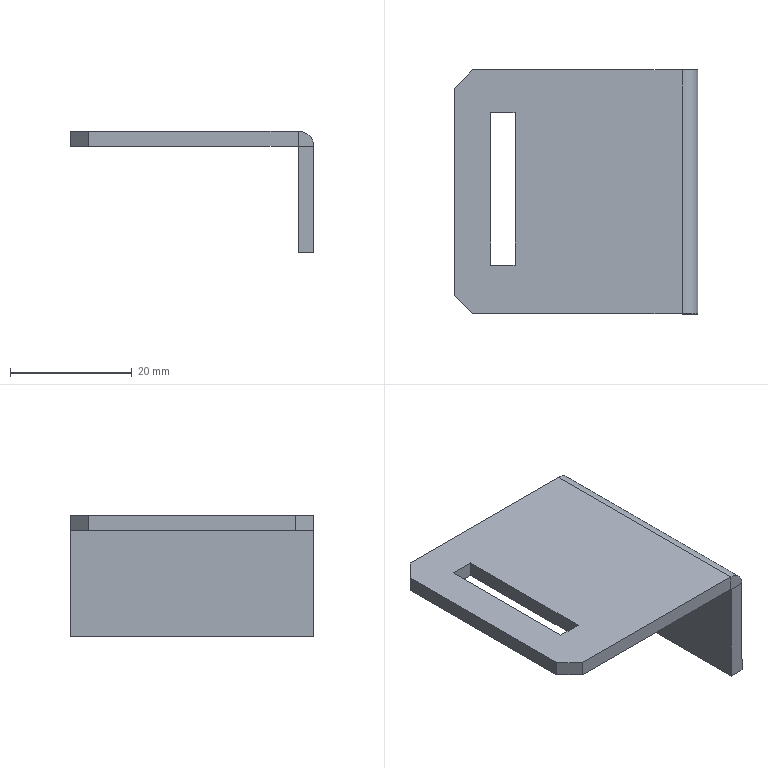Part | SolidWorks | features Chamfer 1, EdgeFlange 1, FlatPattern 1, ICE 1, SMBaseFlange 1, SheetMetal 1 | 1 solid | 20 faces | box 40 x 40 x 20 mm | volume 5420 mm3 | plane 18 | cylinder 2 | commonest cylinder face diameters 0.2 x1 5.2 x1
STEP:
#1=CARTESIAN_POINT('',(-17.,-20.,0.));
#2=VERTEX_POINT('',#1);
#3=CARTESIAN_POINT('',(17.4,-20.,0.));
#4=VERTEX_POINT('',#3);
#5=CARTESIAN_POINT('',(-20.,-20.,0.));
#6=DIRECTION('',(1.,0.,0.));
#7=VECTOR('',#6,1000.);
#8=LINE('',#5,#7);
#9=EDGE_CURVE('',#2,#4,#8,.T.);
#10=ORIENTED_EDGE('',*,*,#9,.F.);
#11=CARTESIAN_POINT('',(-17.,-20.,-2.5));
#12=VERTEX_POINT('',#11);
#13=CARTESIAN_POINT('',(-17.,-20.,-2.5));
#14=DIRECTION('',(0.,0.,-1.));
#15=VECTOR('',#14,1000.);
#16=LINE('',#13,#15);
#17=EDGE_CURVE('',#2,#12,#16,.T.);
#18=ORIENTED_EDGE('',*,*,#17,.T.);
#19=CARTESIAN_POINT('',(17.4,-20.,-2.5));
#20=VERTEX_POINT('',#19);
#21=CARTESIAN_POINT('',(-20.,-20.,-2.5));
#22=DIRECTION('',(1.,0.,0.));
#23=VECTOR('',#22,1000.);
#24=LINE('',#21,#23);
#25=EDGE_CURVE('',#12,#20,#24,.T.);
#26=ORIENTED_EDGE('',*,*,#25,.T.);
#27=CARTESIAN_POINT('',(17.4,-20.,-2.5));
#28=DIRECTION('',(0.,0.,1.));
#29=VECTOR('',#28,1000.);
#30=LINE('',#27,#29);
#31=EDGE_CURVE('',#20,#4,#30,.T.);
#32=ORIENTED_EDGE('',*,*,#31,.T.);
#33=EDGE_LOOP('',(#10,#18,#26,#32));
#34=FACE_OUTER_BOUND('',#33,.T.);
#35=CARTESIAN_POINT('',(-20.,-20.,-2.5));
#36=DIRECTION('',(0.,-1.,0.));
#37=DIRECTION('',(0.,0.,-1.));
#38=AXIS2_PLACEMENT_3D('',#35,#36,#37);
#39=PLANE('',#38);
#40=ADVANCED_FACE('',(#34),#39,.T.);
#41=CARTESIAN_POINT('',(-14.,-12.,-2.5));
#42=VERTEX_POINT('',#41);
#43=CARTESIAN_POINT('',(-10.,-12.,-2.5));
#44=VERTEX_POINT('',#43);
#45=CARTESIAN_POINT('',(0.,-12.,-2.5));
#46=DIRECTION('',(1.,0.,0.));
#47=VECTOR('',#46,1000.);
#48=LINE('',#45,#47);
#49=EDGE_CURVE('',#42,#44,#48,.T.);
#50=ORIENTED_EDGE('',*,*,#49,.T.);
#51=CARTESIAN_POINT('',(-10.,13.,-2.5));
#52=VERTEX_POINT('',#51);
#53=CARTESIAN_POINT('',(-10.,0.,-2.5));
#54=DIRECTION('',(0.,1.,0.));
#55=VECTOR('',#54,1000.);
#56=LINE('',#53,#55);
#57=EDGE_CURVE('',#44,#52,#56,.T.);
#58=ORIENTED_EDGE('',*,*,#57,.T.);
#59=CARTESIAN_POINT('',(-14.,13.,-2.5));
#60=VERTEX_POINT('',#59);
#61=CARTESIAN_POINT('',(0.,13.,-2.5));
#62=DIRECTION('',(-1.,0.,0.));
#63=VECTOR('',#62,1000.);
#64=LINE('',#61,#63);
#65=EDGE_CURVE('',#52,#60,#64,.T.);
#66=ORIENTED_EDGE('',*,*,#65,.T.);
#67=CARTESIAN_POINT('',(-14.,0.,-2.5));
#68=DIRECTION('',(0.,-1.,0.));
#69=VECTOR('',#68,1000.);
#70=LINE('',#67,#69);
#71=EDGE_CURVE('',#60,#42,#70,.T.);
#72=ORIENTED_EDGE('',*,*,#71,.T.);
#73=EDGE_LOOP('',(#50,#58,#66,#72));
#74=FACE_BOUND('',#73,.T.);
#75=CARTESIAN_POINT('',(-20.,17.,-2.5));
#76=VERTEX_POINT('',#75);
#77=CARTESIAN_POINT('',(-20.,-17.,-2.5));
#78=VERTEX_POINT('',#77);
#79=CARTESIAN_POINT('',(-20.,20.,-2.5));
#80=DIRECTION('',(0.,-1.,0.));
#81=VECTOR('',#80,1000.);
#82=LINE('',#79,#81);
#83=EDGE_CURVE('',#76,#78,#82,.T.);
#84=ORIENTED_EDGE('',*,*,#83,.F.);
#85=CARTESIAN_POINT('',(-17.,20.,-2.5));
#86=VERTEX_POINT('',#85);
#87=CARTESIAN_POINT('',(-17.,20.,-2.5));
#88=DIRECTION('',(0.7071,0.7071,0.));
#89=VECTOR('',#88,1000.);
#90=LINE('',#87,#89);
#91=EDGE_CURVE('',#76,#86,#90,.T.);
#92=ORIENTED_EDGE('',*,*,#91,.T.);
#93=CARTESIAN_POINT('',(17.4,20.,-2.5));
#94=VERTEX_POINT('',#93);
#95=CARTESIAN_POINT('',(-20.,20.,-2.5));
#96=DIRECTION('',(-1.,0.,0.));
#97=VECTOR('',#96,1000.);
#98=LINE('',#95,#97);
#99=EDGE_CURVE('',#94,#86,#98,.T.);
#100=ORIENTED_EDGE('',*,*,#99,.F.);
#101=CARTESIAN_POINT('',(17.4,-20.,-2.5));
#102=DIRECTION('',(0.,1.,0.));
#103=VECTOR('',#102,1000.);
#104=LINE('',#101,#103);
#105=EDGE_CURVE('',#20,#94,#104,.T.);
#106=ORIENTED_EDGE('',*,*,#105,.F.);
#107=ORIENTED_EDGE('',*,*,#25,.F.);
#108=CARTESIAN_POINT('',(-20.,-17.,-2.5));
#109=DIRECTION('',(-0.7071,0.7071,0.));
#110=VECTOR('',#109,1000.);
#111=LINE('',#108,#110);
#112=EDGE_CURVE('',#12,#78,#111,.T.);
#113=ORIENTED_EDGE('',*,*,#112,.T.);
#114=EDGE_LOOP('',(#84,#92,#100,#106,#107,#113));
#115=FACE_OUTER_BOUND('',#114,.T.);
#116=CARTESIAN_POINT('',(0.,0.,-2.5));
#117=DIRECTION('',(0.,0.,1.));
#118=DIRECTION('',(1.,0.,0.));
#119=AXIS2_PLACEMENT_3D('',#116,#117,#118);
#120=PLANE('',#119);
#121=ADVANCED_FACE('',(#74,#115),#120,.F.);
#122=CARTESIAN_POINT('',(-10.,-12.,0.));
#123=VERTEX_POINT('',#122);
#124=CARTESIAN_POINT('',(-10.,13.,0.));
#125=VERTEX_POINT('',#124);
#126=CARTESIAN_POINT('',(-10.,13.,0.));
#127=DIRECTION('',(0.,1.,0.));
#128=VECTOR('',#127,1000.);
#129=LINE('',#126,#128);
#130=EDGE_CURVE('',#123,#125,#129,.T.);
#131=ORIENTED_EDGE('',*,*,#130,.F.);
#132=CARTESIAN_POINT('',(-14.,-12.,0.));
#133=VERTEX_POINT('',#132);
#134=CARTESIAN_POINT('',(-14.,-12.,0.));
#135=DIRECTION('',(1.,0.,0.));
#136=VECTOR('',#135,1000.);
#137=LINE('',#134,#136);
#138=EDGE_CURVE('',#133,#123,#137,.T.);
#139=ORIENTED_EDGE('',*,*,#138,.F.);
#140=CARTESIAN_POINT('',(-14.,13.,0.));
#141=VERTEX_POINT('',#140);
#142=CARTESIAN_POINT('',(-14.,13.,0.));
#143=DIRECTION('',(0.,-1.,0.));
#144=VECTOR('',#143,1000.);
#145=LINE('',#142,#144);
#146=EDGE_CURVE('',#141,#133,#145,.T.);
#147=ORIENTED_EDGE('',*,*,#146,.F.);
#148=CARTESIAN_POINT('',(-14.,13.,0.));
#149=DIRECTION('',(-1.,0.,0.));
#150=VECTOR('',#149,1000.);
#151=LINE('',#148,#150);
#152=EDGE_CURVE('',#125,#141,#151,.T.);
#153=ORIENTED_EDGE('',*,*,#152,.F.);
#154=EDGE_LOOP('',(#131,#139,#147,#153));
#155=FACE_BOUND('',#154,.T.);
#156=CARTESIAN_POINT('',(17.4,20.,0.));
#157=VERTEX_POINT('',#156);
#158=CARTESIAN_POINT('',(-17.,20.,0.));
#159=VERTEX_POINT('',#158);
#160=CARTESIAN_POINT('',(-20.,20.,0.));
#161=DIRECTION('',(-1.,0.,0.));
#162=VECTOR('',#161,1000.);
#163=LINE('',#160,#162);
#164=EDGE_CURVE('',#157,#159,#163,.T.);
#165=ORIENTED_EDGE('',*,*,#164,.T.);
#166=CARTESIAN_POINT('',(-20.,17.,0.));
#167=VERTEX_POINT('',#166);
#168=CARTESIAN_POINT('',(-18.5,18.5,0.));
#169=DIRECTION('',(-0.7071,-0.7071,0.));
#170=VECTOR('',#169,1000.);
#171=LINE('',#168,#170);
#172=EDGE_CURVE('',#159,#167,#171,.T.);
#173=ORIENTED_EDGE('',*,*,#172,.T.);
#174=CARTESIAN_POINT('',(-20.,-17.,0.));
#175=VERTEX_POINT('',#174);
#176=CARTESIAN_POINT('',(-20.,20.,0.));
#177=DIRECTION('',(0.,-1.,0.));
#178=VECTOR('',#177,1000.);
#179=LINE('',#176,#178);
#180=EDGE_CURVE('',#167,#175,#179,.T.);
#181=ORIENTED_EDGE('',*,*,#180,.T.);
#182=CARTESIAN_POINT('',(-18.5,-18.5,0.));
#183=DIRECTION('',(0.7071,-0.7071,0.));
#184=VECTOR('',#183,1000.);
#185=LINE('',#182,#184);
#186=EDGE_CURVE('',#175,#2,#185,.T.);
#187=ORIENTED_EDGE('',*,*,#186,.T.);
#188=ORIENTED_EDGE('',*,*,#9,.T.);
#189=CARTESIAN_POINT('',(17.4,-20.,0.));
#190=DIRECTION('',(0.,1.,0.));
#191=VECTOR('',#190,1000.);
#192=LINE('',#189,#191);
#193=EDGE_CURVE('',#4,#157,#192,.T.);
#194=ORIENTED_EDGE('',*,*,#193,.T.);
#195=EDGE_LOOP('',(#165,#173,#181,#187,#188,#194));
#196=FACE_OUTER_BOUND('',#195,.T.);
#197=CARTESIAN_POINT('',(0.,0.,0.));
#198=DIRECTION('',(0.,0.,1.));
#199=DIRECTION('',(1.,0.,0.));
#200=AXIS2_PLACEMENT_3D('',#197,#198,#199);
#201=PLANE('',#200);
#202=ADVANCED_FACE('',(#155,#196),#201,.T.);
#203=ORIENTED_EDGE('',*,*,#180,.F.);
#204=CARTESIAN_POINT('',(-20.,17.,-2.5));
#205=DIRECTION('',(0.,0.,-1.));
#206=VECTOR('',#205,1000.);
#207=LINE('',#204,#206);
#208=EDGE_CURVE('',#167,#76,#207,.T.);
#209=ORIENTED_EDGE('',*,*,#208,.T.);
#210=ORIENTED_EDGE('',*,*,#83,.T.);
#211=CARTESIAN_POINT('',(-20.,-17.,-2.5));
#212=DIRECTION('',(0.,0.,1.));
#213=VECTOR('',#212,1000.);
#214=LINE('',#211,#213);
#215=EDGE_CURVE('',#78,#175,#214,.T.);
#216=ORIENTED_EDGE('',*,*,#215,.T.);
#217=EDGE_LOOP('',(#203,#209,#210,#216));
#218=FACE_OUTER_BOUND('',#217,.T.);
#219=CARTESIAN_POINT('',(-20.,20.,-2.5));
#220=DIRECTION('',(-1.,0.,0.));
#221=DIRECTION('',(0.,0.,1.));
#222=AXIS2_PLACEMENT_3D('',#219,#220,#221);
#223=PLANE('',#222);
#224=ADVANCED_FACE('',(#218),#223,.T.);
#225=ORIENTED_EDGE('',*,*,#99,.T.);
#226=CARTESIAN_POINT('',(-17.,20.,-2.5));
#227=DIRECTION('',(0.,0.,1.));
#228=VECTOR('',#227,1000.);
#229=LINE('',#226,#228);
#230=EDGE_CURVE('',#86,#159,#229,.T.);
#231=ORIENTED_EDGE('',*,*,#230,.T.);
#232=ORIENTED_EDGE('',*,*,#164,.F.);
#233=CARTESIAN_POINT('',(17.4,20.,-2.5));
#234=DIRECTION('',(0.,0.,1.));
#235=VECTOR('',#234,1000.);
#236=LINE('',#233,#235);
#237=EDGE_CURVE('',#94,#157,#236,.T.);
#238=ORIENTED_EDGE('',*,*,#237,.F.);
#239=EDGE_LOOP('',(#225,#231,#232,#238));
#240=FACE_OUTER_BOUND('',#239,.T.);
#241=CARTESIAN_POINT('',(-20.,20.,-2.5));
#242=DIRECTION('',(0.,1.,0.));
#243=DIRECTION('',(0.,0.,1.));
#244=AXIS2_PLACEMENT_3D('',#241,#242,#243);
#245=PLANE('',#244);
#246=ADVANCED_FACE('',(#240),#245,.T.);
#247=CARTESIAN_POINT('',(17.5,20.,-2.6));
#248=VERTEX_POINT('',#247);
#249=CARTESIAN_POINT('',(20.,20.,-2.6));
#250=VERTEX_POINT('',#249);
#251=CARTESIAN_POINT('',(20.,20.,-2.6));
#252=DIRECTION('',(1.,0.,0.));
#253=VECTOR('',#252,1000.);
#254=LINE('',#251,#253);
#255=EDGE_CURVE('',#248,#250,#254,.T.);
#256=ORIENTED_EDGE('',*,*,#255,.F.);
#257=CARTESIAN_POINT('',(17.4,20.,-2.6));
#258=DIRECTION('',(0.,1.,0.));
#259=DIRECTION('',(0.,0.,-1.));
#260=AXIS2_PLACEMENT_3D('',#257,#258,#259);
#261=CIRCLE('',#260,0.1);
#262=EDGE_CURVE('',#94,#248,#261,.T.);
#263=ORIENTED_EDGE('',*,*,#262,.F.);
#264=ORIENTED_EDGE('',*,*,#237,.T.);
#265=CARTESIAN_POINT('',(17.4,20.,-2.6));
#266=DIRECTION('',(0.,1.,0.));
#267=DIRECTION('',(0.,0.,-1.));
#268=AXIS2_PLACEMENT_3D('',#265,#266,#267);
#269=CIRCLE('',#268,2.6);
#270=EDGE_CURVE('',#157,#250,#269,.T.);
#271=ORIENTED_EDGE('',*,*,#270,.T.);
#272=EDGE_LOOP('',(#256,#263,#264,#271));
#273=FACE_OUTER_BOUND('',#272,.T.);
#274=CARTESIAN_POINT('',(17.4,20.,-2.6));
#275=DIRECTION('',(0.,1.,0.));
#276=DIRECTION('',(0.,0.,1.));
#277=AXIS2_PLACEMENT_3D('',#274,#275,#276);
#278=PLANE('',#277);
#279=ADVANCED_FACE('',(#273),#278,.T.);
#280=CARTESIAN_POINT('',(17.5,-20.,-2.6));
#281=VERTEX_POINT('',#280);
#282=CARTESIAN_POINT('',(17.4,-20.,-2.6));
#283=DIRECTION('',(0.,-1.,0.));
#284=DIRECTION('',(0.,0.,-1.));
#285=AXIS2_PLACEMENT_3D('',#282,#283,#284);
#286=CIRCLE('',#285,0.1);
#287=EDGE_CURVE('',#281,#20,#286,.T.);
#288=ORIENTED_EDGE('',*,*,#287,.F.);
#289=CARTESIAN_POINT('',(20.,-20.,-2.6));
#290=VERTEX_POINT('',#289);
#291=CARTESIAN_POINT('',(17.5,-20.,-2.6));
#292=DIRECTION('',(1.,0.,0.));
#293=VECTOR('',#292,1000.);
#294=LINE('',#291,#293);
#295=EDGE_CURVE('',#281,#290,#294,.T.);
#296=ORIENTED_EDGE('',*,*,#295,.T.);
#297=CARTESIAN_POINT('',(17.4,-20.,-2.6));
#298=DIRECTION('',(0.,-1.,0.));
#299=DIRECTION('',(0.,0.,-1.));
#300=AXIS2_PLACEMENT_3D('',#297,#298,#299);
#301=CIRCLE('',#300,2.6);
#302=EDGE_CURVE('',#290,#4,#301,.T.);
#303=ORIENTED_EDGE('',*,*,#302,.T.);
#304=ORIENTED_EDGE('',*,*,#31,.F.);
#305=EDGE_LOOP('',(#288,#296,#303,#304));
#306=FACE_OUTER_BOUND('',#305,.T.);
#307=CARTESIAN_POINT('',(17.4,-20.,-2.6));
#308=DIRECTION('',(0.,1.,0.));
#309=DIRECTION('',(0.,0.,1.));
#310=AXIS2_PLACEMENT_3D('',#307,#308,#309);
#311=PLANE('',#310);
#312=ADVANCED_FACE('',(#306),#311,.F.);
#313=ORIENTED_EDGE('',*,*,#193,.F.);
#314=ORIENTED_EDGE('',*,*,#302,.F.);
#315=CARTESIAN_POINT('',(20.,0.,-2.6));
#316=DIRECTION('',(0.,-1.,0.));
#317=VECTOR('',#316,1000.);
#318=LINE('',#315,#317);
#319=EDGE_CURVE('',#250,#290,#318,.T.);
#320=ORIENTED_EDGE('',*,*,#319,.F.);
#321=ORIENTED_EDGE('',*,*,#270,.F.);
#322=EDGE_LOOP('',(#313,#314,#320,#321));
#323=FACE_OUTER_BOUND('',#322,.T.);
#324=CARTESIAN_POINT('',(17.4,-20.,-2.6));
#325=DIRECTION('',(0.,-1.,0.));
#326=DIRECTION('',(1.,0.,0.));
#327=AXIS2_PLACEMENT_3D('',#324,#325,#326);
#328=CYLINDRICAL_SURFACE('',#327,2.6);
#329=ADVANCED_FACE('',(#323),#328,.T.);
#330=ORIENTED_EDGE('',*,*,#105,.T.);
#331=ORIENTED_EDGE('',*,*,#262,.T.);
#332=CARTESIAN_POINT('',(17.5,20.,-2.6));
#333=DIRECTION('',(0.,-1.,0.));
#334=VECTOR('',#333,1000.);
#335=LINE('',#332,#334);
#336=EDGE_CURVE('',#248,#281,#335,.T.);
#337=ORIENTED_EDGE('',*,*,#336,.T.);
#338=ORIENTED_EDGE('',*,*,#287,.T.);
#339=EDGE_LOOP('',(#330,#331,#337,#338));
#340=FACE_OUTER_BOUND('',#339,.T.);
#341=CARTESIAN_POINT('',(17.4,-20.,-2.6));
#342=DIRECTION('',(0.,-1.,0.));
#343=DIRECTION('',(1.,0.,0.));
#344=AXIS2_PLACEMENT_3D('',#341,#342,#343);
#345=CYLINDRICAL_SURFACE('',#344,0.1);
#346=ADVANCED_FACE('',(#340),#345,.F.);
#347=CARTESIAN_POINT('',(20.,-20.,-20.));
#348=VERTEX_POINT('',#347);
#349=CARTESIAN_POINT('',(20.,-20.,-2.5));
#350=DIRECTION('',(0.,0.,1.));
#351=VECTOR('',#350,1000.);
#352=LINE('',#349,#351);
#353=EDGE_CURVE('',#348,#290,#352,.T.);
#354=ORIENTED_EDGE('',*,*,#353,.T.);
#355=ORIENTED_EDGE('',*,*,#295,.F.);
#356=CARTESIAN_POINT('',(17.5,-20.,-20.));
#357=VERTEX_POINT('',#356);
#358=CARTESIAN_POINT('',(17.5,-20.,0.));
#359=DIRECTION('',(0.,0.,1.));
#360=VECTOR('',#359,1000.);
#361=LINE('',#358,#360);
#362=EDGE_CURVE('',#357,#281,#361,.T.);
#363=ORIENTED_EDGE('',*,*,#362,.F.);
#364=CARTESIAN_POINT('',(20.,-20.,-20.));
#365=DIRECTION('',(-1.,0.,0.));
#366=VECTOR('',#365,1000.);
#367=LINE('',#364,#366);
#368=EDGE_CURVE('',#348,#357,#367,.T.);
#369=ORIENTED_EDGE('',*,*,#368,.F.);
#370=EDGE_LOOP('',(#354,#355,#363,#369));
#371=FACE_OUTER_BOUND('',#370,.T.);
#372=CARTESIAN_POINT('',(20.,-20.,-2.5));
#373=DIRECTION('',(0.,-1.,0.));
#374=DIRECTION('',(0.,0.,-1.));
#375=AXIS2_PLACEMENT_3D('',#372,#373,#374);
#376=PLANE('',#375);
#377=ADVANCED_FACE('',(#371),#376,.T.);
#378=CARTESIAN_POINT('',(17.5,20.,-20.));
#379=VERTEX_POINT('',#378);
#380=CARTESIAN_POINT('',(17.5,20.,0.));
#381=DIRECTION('',(0.,0.,-1.));
#382=VECTOR('',#381,1000.);
#383=LINE('',#380,#382);
#384=EDGE_CURVE('',#248,#379,#383,.T.);
#385=ORIENTED_EDGE('',*,*,#384,.F.);
#386=ORIENTED_EDGE('',*,*,#255,.T.);
#387=CARTESIAN_POINT('',(20.,20.,-20.));
#388=VERTEX_POINT('',#387);
#389=CARTESIAN_POINT('',(20.,20.,-20.));
#390=DIRECTION('',(0.,0.,-1.));
#391=VECTOR('',#390,1000.);
#392=LINE('',#389,#391);
#393=EDGE_CURVE('',#250,#388,#392,.T.);
#394=ORIENTED_EDGE('',*,*,#393,.T.);
#395=CARTESIAN_POINT('',(20.,20.,-20.));
#396=DIRECTION('',(-1.,0.,0.));
#397=VECTOR('',#396,1000.);
#398=LINE('',#395,#397);
#399=EDGE_CURVE('',#388,#379,#398,.T.);
#400=ORIENTED_EDGE('',*,*,#399,.T.);
#401=EDGE_LOOP('',(#385,#386,#394,#400));
#402=FACE_OUTER_BOUND('',#401,.T.);
#403=CARTESIAN_POINT('',(20.,20.,-20.));
#404=DIRECTION('',(0.,1.,0.));
#405=DIRECTION('',(0.,0.,1.));
#406=AXIS2_PLACEMENT_3D('',#403,#404,#405);
#407=PLANE('',#406);
#408=ADVANCED_FACE('',(#402),#407,.T.);
#409=ORIENTED_EDGE('',*,*,#393,.F.);
#410=ORIENTED_EDGE('',*,*,#319,.T.);
#411=ORIENTED_EDGE('',*,*,#353,.F.);
#412=CARTESIAN_POINT('',(20.,-20.,-20.));
#413=DIRECTION('',(0.,-1.,0.));
#414=VECTOR('',#413,1000.);
#415=LINE('',#412,#414);
#416=EDGE_CURVE('',#388,#348,#415,.T.);
#417=ORIENTED_EDGE('',*,*,#416,.F.);
#418=EDGE_LOOP('',(#409,#410,#411,#417));
#419=FACE_OUTER_BOUND('',#418,.T.);
#420=CARTESIAN_POINT('',(20.,0.,0.));
#421=DIRECTION('',(1.,0.,0.));
#422=DIRECTION('',(0.,0.,-1.));
#423=AXIS2_PLACEMENT_3D('',#420,#421,#422);
#424=PLANE('',#423);
#425=ADVANCED_FACE('',(#419),#424,.T.);
#426=ORIENTED_EDGE('',*,*,#336,.F.);
#427=ORIENTED_EDGE('',*,*,#384,.T.);
#428=CARTESIAN_POINT('',(17.5,0.,-20.));
#429=DIRECTION('',(0.,-1.,0.));
#430=VECTOR('',#429,1000.);
#431=LINE('',#428,#430);
#432=EDGE_CURVE('',#379,#357,#431,.T.);
#433=ORIENTED_EDGE('',*,*,#432,.T.);
#434=ORIENTED_EDGE('',*,*,#362,.T.);
#435=EDGE_LOOP('',(#426,#427,#433,#434));
#436=FACE_OUTER_BOUND('',#435,.T.);
#437=CARTESIAN_POINT('',(17.5,0.,0.));
#438=DIRECTION('',(1.,0.,0.));
#439=DIRECTION('',(0.,0.,-1.));
#440=AXIS2_PLACEMENT_3D('',#437,#438,#439);
#441=PLANE('',#440);
#442=ADVANCED_FACE('',(#436),#441,.F.);
#443=ORIENTED_EDGE('',*,*,#432,.F.);
#444=ORIENTED_EDGE('',*,*,#399,.F.);
#445=ORIENTED_EDGE('',*,*,#416,.T.);
#446=ORIENTED_EDGE('',*,*,#368,.T.);
#447=EDGE_LOOP('',(#443,#444,#445,#446));
#448=FACE_OUTER_BOUND('',#447,.T.);
#449=CARTESIAN_POINT('',(20.,-20.,-20.));
#450=DIRECTION('',(0.,0.,-1.));
#451=DIRECTION('',(-1.,0.,0.));
#452=AXIS2_PLACEMENT_3D('',#449,#450,#451);
#453=PLANE('',#452);
#454=ADVANCED_FACE('',(#448),#453,.T.);
#455=CARTESIAN_POINT('',(-10.,-12.,-10.));
#456=DIRECTION('',(0.,0.,1.));
#457=VECTOR('',#456,1000.);
#458=LINE('',#455,#457);
#459=EDGE_CURVE('',#44,#123,#458,.T.);
#460=ORIENTED_EDGE('',*,*,#459,.T.);
#461=ORIENTED_EDGE('',*,*,#130,.T.);
#462=CARTESIAN_POINT('',(-10.,13.,-10.));
#463=DIRECTION('',(0.,0.,1.));
#464=VECTOR('',#463,1000.);
#465=LINE('',#462,#464);
#466=EDGE_CURVE('',#52,#125,#465,.T.);
#467=ORIENTED_EDGE('',*,*,#466,.F.);
#468=ORIENTED_EDGE('',*,*,#57,.F.);
#469=EDGE_LOOP('',(#460,#461,#467,#468));
#470=FACE_OUTER_BOUND('',#469,.T.);
#471=CARTESIAN_POINT('',(-10.,13.,-10.));
#472=DIRECTION('',(1.,0.,0.));
#473=DIRECTION('',(0.,1.,0.));
#474=AXIS2_PLACEMENT_3D('',#471,#472,#473);
#475=PLANE('',#474);
#476=ADVANCED_FACE('',(#470),#475,.F.);
#477=CARTESIAN_POINT('',(-14.,-12.,-10.));
#478=DIRECTION('',(0.,0.,1.));
#479=VECTOR('',#478,1000.);
#480=LINE('',#477,#479);
#481=EDGE_CURVE('',#42,#133,#480,.T.);
#482=ORIENTED_EDGE('',*,*,#481,.T.);
#483=ORIENTED_EDGE('',*,*,#138,.T.);
#484=ORIENTED_EDGE('',*,*,#459,.F.);
#485=ORIENTED_EDGE('',*,*,#49,.F.);
#486=EDGE_LOOP('',(#482,#483,#484,#485));
#487=FACE_OUTER_BOUND('',#486,.T.);
#488=CARTESIAN_POINT('',(-14.,-12.,-10.));
#489=DIRECTION('',(0.,-1.,0.));
#490=DIRECTION('',(0.,0.,-1.));
#491=AXIS2_PLACEMENT_3D('',#488,#489,#490);
#492=PLANE('',#491);
#493=ADVANCED_FACE('',(#487),#492,.F.);
#494=CARTESIAN_POINT('',(-14.,13.,-10.));
#495=DIRECTION('',(0.,0.,1.));
#496=VECTOR('',#495,1000.);
#497=LINE('',#494,#496);
#498=EDGE_CURVE('',#60,#141,#497,.T.);
#499=ORIENTED_EDGE('',*,*,#498,.T.);
#500=ORIENTED_EDGE('',*,*,#146,.T.);
#501=ORIENTED_EDGE('',*,*,#481,.F.);
#502=ORIENTED_EDGE('',*,*,#71,.F.);
#503=EDGE_LOOP('',(#499,#500,#501,#502));
#504=FACE_OUTER_BOUND('',#503,.T.);
#505=CARTESIAN_POINT('',(-14.,13.,-10.));
#506=DIRECTION('',(-1.,0.,0.));
#507=DIRECTION('',(0.,-1.,0.));
#508=AXIS2_PLACEMENT_3D('',#505,#506,#507);
#509=PLANE('',#508);
#510=ADVANCED_FACE('',(#504),#509,.F.);
#511=ORIENTED_EDGE('',*,*,#466,.T.);
#512=ORIENTED_EDGE('',*,*,#152,.T.);
#513=ORIENTED_EDGE('',*,*,#498,.F.);
#514=ORIENTED_EDGE('',*,*,#65,.F.);
#515=EDGE_LOOP('',(#511,#512,#513,#514));
#516=FACE_OUTER_BOUND('',#515,.T.);
#517=CARTESIAN_POINT('',(-14.,13.,-10.));
#518=DIRECTION('',(0.,1.,0.));
#519=DIRECTION('',(-1.,0.,0.));
#520=AXIS2_PLACEMENT_3D('',#517,#518,#519);
#521=PLANE('',#520);
#522=ADVANCED_FACE('',(#516),#521,.F.);
#523=ORIENTED_EDGE('',*,*,#91,.F.);
#524=ORIENTED_EDGE('',*,*,#208,.F.);
#525=ORIENTED_EDGE('',*,*,#172,.F.);
#526=ORIENTED_EDGE('',*,*,#230,.F.);
#527=EDGE_LOOP('',(#523,#524,#525,#526));
#528=FACE_OUTER_BOUND('',#527,.T.);
#529=CARTESIAN_POINT('',(-17.,20.,-2.5));
#530=DIRECTION('',(0.7071,-0.7071,0.));
#531=DIRECTION('',(0.,0.,1.));
#532=AXIS2_PLACEMENT_3D('',#529,#530,#531);
#533=PLANE('',#532);
#534=ADVANCED_FACE('',(#528),#533,.F.);
#535=ORIENTED_EDGE('',*,*,#112,.F.);
#536=ORIENTED_EDGE('',*,*,#17,.F.);
#537=ORIENTED_EDGE('',*,*,#186,.F.);
#538=ORIENTED_EDGE('',*,*,#215,.F.);
#539=EDGE_LOOP('',(#535,#536,#537,#538));
#540=FACE_OUTER_BOUND('',#539,.T.);
#541=CARTESIAN_POINT('',(-20.,-17.,-2.5));
#542=DIRECTION('',(0.7071,0.7071,0.));
#543=DIRECTION('',(0.,0.,1.));
#544=AXIS2_PLACEMENT_3D('',#541,#542,#543);
#545=PLANE('',#544);
#546=ADVANCED_FACE('',(#540),#545,.F.);
#547=CLOSED_SHELL('',(#40,#121,#202,#224,#246,#279,#312,#329,#346,#377,#408,#425,#442,#454,#476,#493,#510,#522,#534,#546));
#548=MANIFOLD_SOLID_BREP('',#547);
#549=CARTESIAN_POINT('',(0.,0.,0.));
#550=DIRECTION('',(0.,0.,1.));
#551=DIRECTION('',(1.,0.,0.));
#552=AXIS2_PLACEMENT_3D('',#549,#550,#551);
#553=(LENGTH_UNIT()NAMED_UNIT(*)SI_UNIT(.MILLI.,.METRE.));
#554=UNCERTAINTY_MEASURE_WITH_UNIT(LENGTH_MEASURE(0.00001),#553,'','');
#555=(NAMED_UNIT(*)PLANE_ANGLE_UNIT()SI_UNIT($,.RADIAN.));
#556=(NAMED_UNIT(*)SI_UNIT($,.STERADIAN.)SOLID_ANGLE_UNIT());
#557=(GEOMETRIC_REPRESENTATION_CONTEXT(3)GLOBAL_UNCERTAINTY_ASSIGNED_CONTEXT((#554))GLOBAL_UNIT_ASSIGNED_CONTEXT((#553,#555,#556))REPRESENTATION_CONTEXT('',''));
#558=ADVANCED_BREP_SHAPE_REPRESENTATION('',(#548,#552),#557);